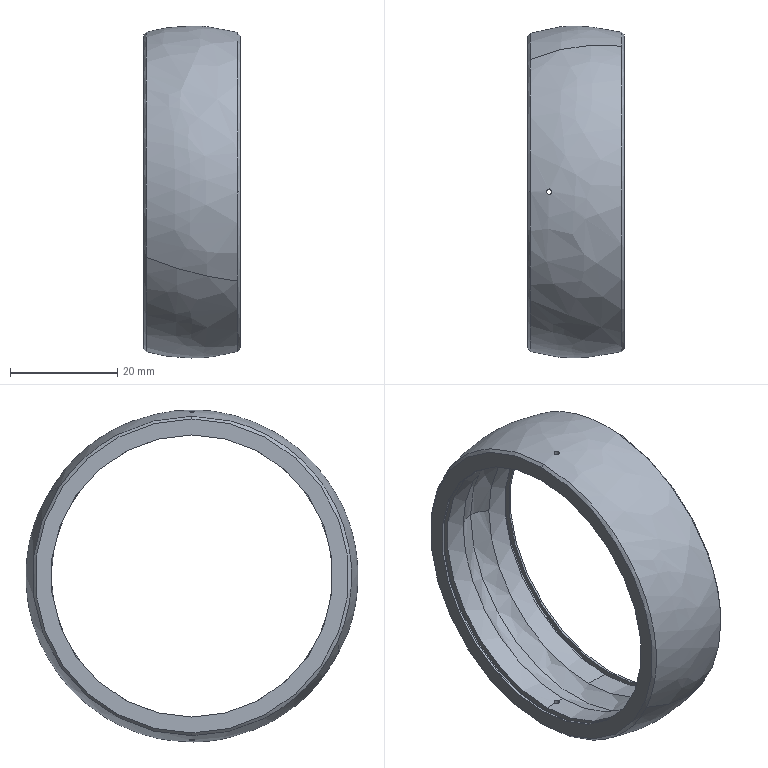Part | SolidWorks | features BaseBody 1 | 1 solid | 32 faces | box 18 x 62 x 62 mm | volume 12092 mm3 | cylinder 16 | spline 6 | plane 6 | cone 4 | commonest cylinder face diameters 52.667 x8 1 x4 54.667 x4
STEP:
#1=CARTESIAN_POINT('',(-5.,62.5,12.31));
#2=VERTEX_POINT('',#1);
#3=CARTESIAN_POINT('',(-5.,63.5,12.31));
#4=VERTEX_POINT('',#3);
#5=CARTESIAN_POINT('',(-5.,62.5,12.31));
#6=CARTESIAN_POINT('',(-4.87,62.5,12.289));
#7=CARTESIAN_POINT('',(-4.741,62.552,12.268));
#8=CARTESIAN_POINT('',(-4.554,62.738,12.237));
#9=CARTESIAN_POINT('',(-4.5,62.867,12.228));
#10=CARTESIAN_POINT('',(-4.5,63.133,12.228));
#11=CARTESIAN_POINT('',(-4.555,63.263,12.237));
#12=CARTESIAN_POINT('',(-4.74,63.447,12.268));
#13=CARTESIAN_POINT('',(-4.87,63.5,12.289));
#14=CARTESIAN_POINT('',(-5.,63.5,12.31));
#15=B_SPLINE_CURVE_WITH_KNOTS('',3,(#5,#6,#7,#8,#9,#10,#11,#12,#13,#14),.UNSPECIFIED.,.F.,.F.,(4,2,2,2,4),(0.000787,0.00118,0.001574,0.001967,0.00236),.UNSPECIFIED.);
#16=EDGE_CURVE('',#2,#4,#15,.T.);
#17=ORIENTED_EDGE('',*,*,#16,.T.);
#18=CARTESIAN_POINT('',(-5.,63.5,12.31));
#19=CARTESIAN_POINT('',(-5.13,63.5,12.331));
#20=CARTESIAN_POINT('',(-5.259,63.448,12.352));
#21=CARTESIAN_POINT('',(-5.446,63.262,12.383));
#22=CARTESIAN_POINT('',(-5.5,63.133,12.392));
#23=CARTESIAN_POINT('',(-5.5,62.867,12.392));
#24=CARTESIAN_POINT('',(-5.445,62.737,12.383));
#25=CARTESIAN_POINT('',(-5.26,62.553,12.352));
#26=CARTESIAN_POINT('',(-5.13,62.5,12.331));
#27=CARTESIAN_POINT('',(-5.,62.5,12.31));
#28=B_SPLINE_CURVE_WITH_KNOTS('',3,(#18,#19,#20,#21,#22,#23,#24,#25,#26,#27),.UNSPECIFIED.,.F.,.F.,(4,2,2,2,4),(0.00236,0.002754,0.003147,0.003541,0.003934),.UNSPECIFIED.);
#29=EDGE_CURVE('',#4,#2,#28,.T.);
#30=ORIENTED_EDGE('',*,*,#29,.T.);
#31=EDGE_LOOP('',(#17,#30));
#32=FACE_BOUND('',#31,.T.);
#33=CARTESIAN_POINT('',(8.5,92.812,42.9));
#34=VERTEX_POINT('',#33);
#35=CARTESIAN_POINT('',(8.5,38.269,26.252));
#36=VERTEX_POINT('',#35);
#37=CARTESIAN_POINT('',(8.5,63.,42.9));
#38=DIRECTION('',(-1.,0.,0.));
#39=DIRECTION('',(0.,0.,1.));
#40=AXIS2_PLACEMENT_3D('',#37,#38,#39);
#41=CIRCLE('',#40,29.812);
#42=EDGE_CURVE('',#34,#36,#41,.T.);
#43=ORIENTED_EDGE('',*,*,#42,.T.);
#44=CARTESIAN_POINT('',(-8.5,35.801,30.694));
#45=VERTEX_POINT('',#44);
#46=CARTESIAN_POINT('',(0.,63.,42.9));
#47=DIRECTION('',(-0.2864,0.4654,-0.8375));
#48=DIRECTION('',(0.7936,0.605,0.06481));
#49=AXIS2_PLACEMENT_3D('',#46,#47,#48);
#50=CIRCLE('',#49,31.);
#51=EDGE_CURVE('',#36,#45,#50,.T.);
#52=ORIENTED_EDGE('',*,*,#51,.T.);
#53=CARTESIAN_POINT('',(-8.5,63.,13.088));
#54=VERTEX_POINT('',#53);
#55=CARTESIAN_POINT('',(-8.5,63.,42.9));
#56=DIRECTION('',(1.,0.,0.));
#57=DIRECTION('',(0.,1.,0.));
#58=AXIS2_PLACEMENT_3D('',#55,#56,#57);
#59=CIRCLE('',#58,29.812);
#60=EDGE_CURVE('',#45,#54,#59,.T.);
#61=ORIENTED_EDGE('',*,*,#60,.T.);
#62=CARTESIAN_POINT('',(-8.5,87.731,59.548));
#63=VERTEX_POINT('',#62);
#64=CARTESIAN_POINT('',(-8.5,63.,42.9));
#65=DIRECTION('',(1.,0.,0.));
#66=DIRECTION('',(0.,1.,0.));
#67=AXIS2_PLACEMENT_3D('',#64,#65,#66);
#68=CIRCLE('',#67,29.812);
#69=EDGE_CURVE('',#54,#63,#68,.T.);
#70=ORIENTED_EDGE('',*,*,#69,.T.);
#71=CARTESIAN_POINT('',(8.5,90.199,55.106));
#72=VERTEX_POINT('',#71);
#73=CARTESIAN_POINT('',(0.,63.,42.9));
#74=DIRECTION('',(0.2864,-0.4654,0.8375));
#75=DIRECTION('',(0.7936,0.605,0.06481));
#76=AXIS2_PLACEMENT_3D('',#73,#74,#75);
#77=CIRCLE('',#76,31.);
#78=EDGE_CURVE('',#72,#63,#77,.T.);
#79=ORIENTED_EDGE('',*,*,#78,.F.);
#80=CARTESIAN_POINT('',(8.5,63.,42.9));
#81=DIRECTION('',(-1.,0.,0.));
#82=DIRECTION('',(0.,0.,1.));
#83=AXIS2_PLACEMENT_3D('',#80,#81,#82);
#84=CIRCLE('',#83,29.812);
#85=EDGE_CURVE('',#72,#34,#84,.T.);
#86=ORIENTED_EDGE('',*,*,#85,.T.);
#87=EDGE_LOOP('',(#43,#52,#61,#70,#79,#86));
#88=FACE_OUTER_BOUND('',#87,.T.);
#89=CARTESIAN_POINT('',(29.685,66.413,34.646));
#90=CARTESIAN_POINT('',(19.256,83.361,4.143));
#91=CARTESIAN_POINT('',(-0.2971,106.892,23.903));
#92=CARTESIAN_POINT('',(10.133,89.943,54.406));
#93=CARTESIAN_POINT('',(28.979,46.842,24.013));
#94=CARTESIAN_POINT('',(8.22,80.575,-36.698));
#95=CARTESIAN_POINT('',(-30.696,127.408,2.631));
#96=CARTESIAN_POINT('',(-9.938,93.675,63.342));
#97=CARTESIAN_POINT('',(11.581,33.025,22.285));
#98=CARTESIAN_POINT('',(-9.478,67.245,-39.303));
#99=CARTESIAN_POINT('',(-48.957,114.755,0.5944));
#100=CARTESIAN_POINT('',(-27.898,80.535,62.182));
#101=CARTESIAN_POINT('',(-8.81,35.843,30.823));
#102=CARTESIAN_POINT('',(-19.903,53.869,-1.621));
#103=CARTESIAN_POINT('',(-40.7,78.897,19.396));
#104=CARTESIAN_POINT('',(-29.606,60.87,51.84));
#105=(BOUNDED_SURFACE()B_SPLINE_SURFACE(3,3,((#89,#90,#91,#92),(#93,#94,#95,#96),(#97,#98,#99,#100),(#101,#102,#103,#104)),.UNSPECIFIED.,.F.,.F.,.T.)B_SPLINE_SURFACE_WITH_KNOTS((4,4),(4,4),(0.,1.),(0.,1.),.UNSPECIFIED.)GEOMETRIC_REPRESENTATION_ITEM()RATIONAL_B_SPLINE_SURFACE(((1.,0.3333,0.3333,1.),(0.7375,0.2458,0.2458,0.7375),(0.7375,0.2458,0.2458,0.7375),(1.,0.3333,0.3333,1.)))REPRESENTATION_ITEM('')SURFACE());
#106=ADVANCED_FACE('',(#32,#88),#105,.T.);
#107=CARTESIAN_POINT('',(0.,90.763,42.9));
#108=VERTEX_POINT('',#107);
#109=CARTESIAN_POINT('',(0.,35.238,42.9));
#110=VERTEX_POINT('',#109);
#111=CARTESIAN_POINT('',(0.,63.,42.9));
#112=DIRECTION('',(-1.,0.,0.));
#113=DIRECTION('',(0.,-1.,0.));
#114=AXIS2_PLACEMENT_3D('',#111,#112,#113);
#115=CIRCLE('',#114,27.762);
#116=EDGE_CURVE('',#108,#110,#115,.T.);
#117=ORIENTED_EDGE('',*,*,#116,.F.);
#118=CARTESIAN_POINT('',(-3.401,89.334,42.9));
#119=VERTEX_POINT('',#118);
#120=CARTESIAN_POINT('',(0.,86.,42.9));
#121=DIRECTION('',(0.,0.,1.));
#122=DIRECTION('',(0.,1.,0.));
#123=AXIS2_PLACEMENT_3D('',#120,#121,#122);
#124=CIRCLE('',#123,4.762);
#125=EDGE_CURVE('',#108,#119,#124,.T.);
#126=ORIENTED_EDGE('',*,*,#125,.T.);
#127=CARTESIAN_POINT('',(-3.401,63.,16.566));
#128=VERTEX_POINT('',#127);
#129=CARTESIAN_POINT('',(-3.401,63.,42.9));
#130=DIRECTION('',(1.,0.,0.));
#131=DIRECTION('',(0.,0.,1.));
#132=AXIS2_PLACEMENT_3D('',#129,#130,#131);
#133=CIRCLE('',#132,26.334);
#134=EDGE_CURVE('',#128,#119,#133,.T.);
#135=ORIENTED_EDGE('',*,*,#134,.F.);
#136=CARTESIAN_POINT('',(-3.401,36.666,42.9));
#137=VERTEX_POINT('',#136);
#138=CARTESIAN_POINT('',(-3.401,63.,42.9));
#139=DIRECTION('',(1.,0.,0.));
#140=DIRECTION('',(0.,0.,1.));
#141=AXIS2_PLACEMENT_3D('',#138,#139,#140);
#142=CIRCLE('',#141,26.334);
#143=EDGE_CURVE('',#137,#128,#142,.T.);
#144=ORIENTED_EDGE('',*,*,#143,.F.);
#145=CARTESIAN_POINT('',(0.,40.,42.9));
#146=DIRECTION('',(0.,0.,-1.));
#147=DIRECTION('',(0.,-1.,0.));
#148=AXIS2_PLACEMENT_3D('',#145,#146,#147);
#149=CIRCLE('',#148,4.762);
#150=EDGE_CURVE('',#110,#137,#149,.T.);
#151=ORIENTED_EDGE('',*,*,#150,.F.);
#152=EDGE_LOOP('',(#117,#126,#135,#144,#151));
#153=FACE_OUTER_BOUND('',#152,.T.);
#154=CARTESIAN_POINT('',(0.,90.763,42.9));
#155=CARTESIAN_POINT('',(0.,90.763,-12.625));
#156=CARTESIAN_POINT('',(0.,35.238,-12.625));
#157=CARTESIAN_POINT('',(0.,35.237,42.9));
#158=CARTESIAN_POINT('',(-1.297,90.763,42.9));
#159=CARTESIAN_POINT('',(-1.297,90.763,-12.625));
#160=CARTESIAN_POINT('',(-1.297,35.238,-12.625));
#161=CARTESIAN_POINT('',(-1.297,35.237,42.9));
#162=CARTESIAN_POINT('',(-2.493,90.26,42.9));
#163=CARTESIAN_POINT('',(-2.493,90.26,-11.62));
#164=CARTESIAN_POINT('',(-2.493,35.74,-11.62));
#165=CARTESIAN_POINT('',(-2.493,35.74,42.9));
#166=CARTESIAN_POINT('',(-3.401,89.334,42.9));
#167=CARTESIAN_POINT('',(-3.401,89.334,-9.767));
#168=CARTESIAN_POINT('',(-3.401,36.666,-9.767));
#169=CARTESIAN_POINT('',(-3.401,36.666,42.9));
#170=(BOUNDED_SURFACE()B_SPLINE_SURFACE(3,3,((#154,#155,#156,#157),(#158,#159,#160,#161),(#162,#163,#164,#165),(#166,#167,#168,#169)),.UNSPECIFIED.,.F.,.F.,.F.)B_SPLINE_SURFACE_WITH_KNOTS((4,4),(4,4),(0.,1.),(0.,1.),.UNSPECIFIED.)GEOMETRIC_REPRESENTATION_ITEM()RATIONAL_B_SPLINE_SURFACE(((1.,0.3333,0.3333,1.),(0.948,0.316,0.316,0.948),(0.948,0.316,0.316,0.948),(1.,0.3333,0.3333,1.)))REPRESENTATION_ITEM('')SURFACE());
#171=ADVANCED_FACE('',(#153),#170,.T.);
#172=CARTESIAN_POINT('',(3.401,63.,16.566));
#173=VERTEX_POINT('',#172);
#174=CARTESIAN_POINT('',(3.401,89.334,42.9));
#175=VERTEX_POINT('',#174);
#176=CARTESIAN_POINT('',(3.401,63.,42.9));
#177=DIRECTION('',(1.,0.,0.));
#178=DIRECTION('',(0.,-1.,0.));
#179=AXIS2_PLACEMENT_3D('',#176,#177,#178);
#180=CIRCLE('',#179,26.334);
#181=EDGE_CURVE('',#173,#175,#180,.T.);
#182=ORIENTED_EDGE('',*,*,#181,.T.);
#183=CARTESIAN_POINT('',(0.,86.,42.9));
#184=DIRECTION('',(0.,0.,1.));
#185=DIRECTION('',(0.,1.,0.));
#186=AXIS2_PLACEMENT_3D('',#183,#184,#185);
#187=CIRCLE('',#186,4.762);
#188=EDGE_CURVE('',#175,#108,#187,.T.);
#189=ORIENTED_EDGE('',*,*,#188,.T.);
#190=ORIENTED_EDGE('',*,*,#116,.T.);
#191=CARTESIAN_POINT('',(3.401,36.666,42.9));
#192=VERTEX_POINT('',#191);
#193=CARTESIAN_POINT('',(0.,40.,42.9));
#194=DIRECTION('',(0.,0.,-1.));
#195=DIRECTION('',(0.,-1.,0.));
#196=AXIS2_PLACEMENT_3D('',#193,#194,#195);
#197=CIRCLE('',#196,4.762);
#198=EDGE_CURVE('',#192,#110,#197,.T.);
#199=ORIENTED_EDGE('',*,*,#198,.F.);
#200=CARTESIAN_POINT('',(3.401,63.,42.9));
#201=DIRECTION('',(1.,0.,0.));
#202=DIRECTION('',(0.,-1.,0.));
#203=AXIS2_PLACEMENT_3D('',#200,#201,#202);
#204=CIRCLE('',#203,26.334);
#205=EDGE_CURVE('',#192,#173,#204,.T.);
#206=ORIENTED_EDGE('',*,*,#205,.T.);
#207=EDGE_LOOP('',(#182,#189,#190,#199,#206));
#208=FACE_OUTER_BOUND('',#207,.T.);
#209=CARTESIAN_POINT('',(3.401,89.334,42.9));
#210=CARTESIAN_POINT('',(3.401,89.334,-9.767));
#211=CARTESIAN_POINT('',(3.401,36.666,-9.767));
#212=CARTESIAN_POINT('',(3.401,36.666,42.9));
#213=CARTESIAN_POINT('',(2.493,90.26,42.9));
#214=CARTESIAN_POINT('',(2.493,90.26,-11.62));
#215=CARTESIAN_POINT('',(2.493,35.74,-11.62));
#216=CARTESIAN_POINT('',(2.493,35.74,42.9));
#217=CARTESIAN_POINT('',(1.297,90.763,42.9));
#218=CARTESIAN_POINT('',(1.297,90.763,-12.625));
#219=CARTESIAN_POINT('',(1.297,35.237,-12.625));
#220=CARTESIAN_POINT('',(1.297,35.237,42.9));
#221=CARTESIAN_POINT('',(0.,90.763,42.9));
#222=CARTESIAN_POINT('',(0.,90.763,-12.625));
#223=CARTESIAN_POINT('',(0.,35.238,-12.625));
#224=CARTESIAN_POINT('',(0.,35.237,42.9));
#225=(BOUNDED_SURFACE()B_SPLINE_SURFACE(3,3,((#209,#210,#211,#212),(#213,#214,#215,#216),(#217,#218,#219,#220),(#221,#222,#223,#224)),.UNSPECIFIED.,.F.,.F.,.F.)B_SPLINE_SURFACE_WITH_KNOTS((4,4),(4,4),(0.,1.),(0.,1.),.UNSPECIFIED.)GEOMETRIC_REPRESENTATION_ITEM()RATIONAL_B_SPLINE_SURFACE(((1.,0.3333,0.3333,1.),(0.948,0.316,0.316,0.948),(0.948,0.316,0.316,0.948),(1.,0.3333,0.3333,1.)))REPRESENTATION_ITEM('')SURFACE());
#226=ADVANCED_FACE('',(#208),#225,.T.);
#227=CARTESIAN_POINT('',(-5.,63.5,69.229));
#228=VERTEX_POINT('',#227);
#229=CARTESIAN_POINT('',(-5.5,63.,69.234));
#230=VERTEX_POINT('',#229);
#231=CARTESIAN_POINT('',(-5.,63.5,69.229));
#232=CARTESIAN_POINT('',(-5.132,63.5,69.229));
#233=CARTESIAN_POINT('',(-5.261,63.446,69.23));
#234=CARTESIAN_POINT('',(-5.446,63.262,69.233));
#235=CARTESIAN_POINT('',(-5.5,63.132,69.234));
#236=CARTESIAN_POINT('',(-5.5,63.,69.234));
#237=B_SPLINE_CURVE_WITH_KNOTS('',3,(#231,#232,#233,#234,#235,#236),.UNSPECIFIED.,.F.,.F.,(4,2,4),(0.,0.0003905,0.0007811),.UNSPECIFIED.);
#238=EDGE_CURVE('',#228,#230,#237,.T.);
#239=ORIENTED_EDGE('',*,*,#238,.F.);
#240=CARTESIAN_POINT('',(-5.,63.5,73.49));
#241=VERTEX_POINT('',#240);
#242=CARTESIAN_POINT('',(-5.,63.5,71.565));
#243=DIRECTION('',(0.,0.,1.));
#244=VECTOR('',#243,1000.);
#245=LINE('',#242,#244);
#246=EDGE_CURVE('',#228,#241,#245,.T.);
#247=ORIENTED_EDGE('',*,*,#246,.T.);
#248=CARTESIAN_POINT('',(-5.,62.5,73.49));
#249=VERTEX_POINT('',#248);
#250=CARTESIAN_POINT('',(-5.,62.5,73.49));
#251=CARTESIAN_POINT('',(-5.13,62.5,73.469));
#252=CARTESIAN_POINT('',(-5.259,62.552,73.448));
#253=CARTESIAN_POINT('',(-5.446,62.738,73.417));
#254=CARTESIAN_POINT('',(-5.5,62.867,73.408));
#255=CARTESIAN_POINT('',(-5.5,63.133,73.408));
#256=CARTESIAN_POINT('',(-5.445,63.263,73.417));
#257=CARTESIAN_POINT('',(-5.26,63.447,73.448));
#258=CARTESIAN_POINT('',(-5.13,63.5,73.469));
#259=CARTESIAN_POINT('',(-5.,63.5,73.49));
#260=B_SPLINE_CURVE_WITH_KNOTS('',3,(#250,#251,#252,#253,#254,#255,#256,#257,#258,#259),.UNSPECIFIED.,.F.,.F.,(4,2,2,2,4),(0.000787,0.00118,0.001574,0.001967,0.00236),.UNSPECIFIED.);
#261=EDGE_CURVE('',#249,#241,#260,.T.);
#262=ORIENTED_EDGE('',*,*,#261,.F.);
#263=CARTESIAN_POINT('',(-5.,62.5,69.229));
#264=VERTEX_POINT('',#263);
#265=CARTESIAN_POINT('',(-5.,62.5,71.565));
#266=DIRECTION('',(0.,0.,1.));
#267=VECTOR('',#266,1000.);
#268=LINE('',#265,#267);
#269=EDGE_CURVE('',#264,#249,#268,.T.);
#270=ORIENTED_EDGE('',*,*,#269,.F.);
#271=CARTESIAN_POINT('',(-5.5,63.,69.234));
#272=CARTESIAN_POINT('',(-5.5,62.868,69.234));
#273=CARTESIAN_POINT('',(-5.446,62.739,69.233));
#274=CARTESIAN_POINT('',(-5.262,62.554,69.23));
#275=CARTESIAN_POINT('',(-5.132,62.5,69.229));
#276=CARTESIAN_POINT('',(-5.,62.5,69.229));
#277=B_SPLINE_CURVE_WITH_KNOTS('',3,(#271,#272,#273,#274,#275,#276),.UNSPECIFIED.,.F.,.F.,(4,2,4),(0.0007811,0.001172,0.001562),.UNSPECIFIED.);
#278=EDGE_CURVE('',#230,#264,#277,.T.);
#279=ORIENTED_EDGE('',*,*,#278,.F.);
#280=EDGE_LOOP('',(#239,#247,#262,#270,#279));
#281=FACE_OUTER_BOUND('',#280,.T.);
#282=CARTESIAN_POINT('',(-5.,63.,71.565));
#283=DIRECTION('',(0.,0.,1.));
#284=DIRECTION('',(0.,-1.,0.));
#285=AXIS2_PLACEMENT_3D('',#282,#283,#284);
#286=CYLINDRICAL_SURFACE('',#285,0.5);
#287=ADVANCED_FACE('',(#281),#286,.F.);
#288=CARTESIAN_POINT('',(-9.,63.,13.588));
#289=VERTEX_POINT('',#288);
#290=CARTESIAN_POINT('',(-9.,63.,72.212));
#291=VERTEX_POINT('',#290);
#292=CARTESIAN_POINT('',(-9.,63.,42.9));
#293=DIRECTION('',(1.,0.,0.));
#294=DIRECTION('',(0.,0.,-1.));
#295=AXIS2_PLACEMENT_3D('',#292,#293,#294);
#296=CIRCLE('',#295,29.312);
#297=EDGE_CURVE('',#289,#291,#296,.T.);
#298=ORIENTED_EDGE('',*,*,#297,.T.);
#299=CARTESIAN_POINT('',(-8.5,63.,72.712));
#300=VERTEX_POINT('',#299);
#301=CARTESIAN_POINT('',(-8.5,63.,72.712));
#302=DIRECTION('',(0.7071,0.,0.7071));
#303=VECTOR('',#302,1000.);
#304=LINE('',#301,#303);
#305=EDGE_CURVE('',#291,#300,#304,.T.);
#306=ORIENTED_EDGE('',*,*,#305,.T.);
#307=CARTESIAN_POINT('',(-8.5,63.,42.9));
#308=DIRECTION('',(1.,0.,0.));
#309=DIRECTION('',(0.,1.,0.));
#310=AXIS2_PLACEMENT_3D('',#307,#308,#309);
#311=CIRCLE('',#310,29.812);
#312=EDGE_CURVE('',#63,#300,#311,.T.);
#313=ORIENTED_EDGE('',*,*,#312,.F.);
#314=ORIENTED_EDGE('',*,*,#69,.F.);
#315=CARTESIAN_POINT('',(-8.5,63.,13.088));
#316=DIRECTION('',(0.7071,0.,-0.7071));
#317=VECTOR('',#316,1000.);
#318=LINE('',#315,#317);
#319=EDGE_CURVE('',#289,#54,#318,.T.);
#320=ORIENTED_EDGE('',*,*,#319,.F.);
#321=EDGE_LOOP('',(#298,#306,#313,#314,#320));
#322=FACE_OUTER_BOUND('',#321,.T.);
#323=CARTESIAN_POINT('',(-8.5,63.,42.9));
#324=DIRECTION('',(1.,0.,0.));
#325=DIRECTION('',(0.,0.,-1.));
#326=AXIS2_PLACEMENT_3D('',#323,#324,#325);
#327=CONICAL_SURFACE('',#326,29.812,0.7854);
#328=ADVANCED_FACE('',(#322),#327,.T.);
#329=CARTESIAN_POINT('',(9.,33.688,42.9));
#330=VERTEX_POINT('',#329);
#331=CARTESIAN_POINT('',(9.,92.312,42.9));
#332=VERTEX_POINT('',#331);
#333=CARTESIAN_POINT('',(9.,63.,42.9));
#334=DIRECTION('',(-1.,0.,0.));
#335=DIRECTION('',(0.,-1.,0.));
#336=AXIS2_PLACEMENT_3D('',#333,#334,#335);
#337=CIRCLE('',#336,29.312);
#338=EDGE_CURVE('',#330,#332,#337,.T.);
#339=ORIENTED_EDGE('',*,*,#338,.T.);
#340=CARTESIAN_POINT('',(8.5,92.812,42.9));
#341=DIRECTION('',(-0.7071,0.7071,0.));
#342=VECTOR('',#341,1000.);
#343=LINE('',#340,#342);
#344=EDGE_CURVE('',#332,#34,#343,.T.);
#345=ORIENTED_EDGE('',*,*,#344,.T.);
#346=ORIENTED_EDGE('',*,*,#85,.F.);
#347=CARTESIAN_POINT('',(8.5,33.188,42.9));
#348=VERTEX_POINT('',#347);
#349=CARTESIAN_POINT('',(8.5,63.,42.9));
#350=DIRECTION('',(-1.,0.,0.));
#351=DIRECTION('',(0.,0.,1.));
#352=AXIS2_PLACEMENT_3D('',#349,#350,#351);
#353=CIRCLE('',#352,29.812);
#354=EDGE_CURVE('',#348,#72,#353,.T.);
#355=ORIENTED_EDGE('',*,*,#354,.F.);
#356=CARTESIAN_POINT('',(8.5,33.188,42.9));
#357=DIRECTION('',(-0.7071,-0.7071,0.));
#358=VECTOR('',#357,1000.);
#359=LINE('',#356,#358);
#360=EDGE_CURVE('',#330,#348,#359,.T.);
#361=ORIENTED_EDGE('',*,*,#360,.F.);
#362=EDGE_LOOP('',(#339,#345,#346,#355,#361));
#363=FACE_OUTER_BOUND('',#362,.T.);
#364=CARTESIAN_POINT('',(8.5,63.,42.9));
#365=DIRECTION('',(-1.,0.,0.));
#366=DIRECTION('',(0.,-1.,0.));
#367=AXIS2_PLACEMENT_3D('',#364,#365,#366);
#368=CONICAL_SURFACE('',#367,29.812,0.7854);
#369=ADVANCED_FACE('',(#363),#368,.T.);
#370=CARTESIAN_POINT('',(-3.401,63.,69.234));
#371=VERTEX_POINT('',#370);
#372=CARTESIAN_POINT('',(-3.401,63.,42.9));
#373=DIRECTION('',(1.,0.,0.));
#374=DIRECTION('',(0.,0.,1.));
#375=AXIS2_PLACEMENT_3D('',#372,#373,#374);
#376=CIRCLE('',#375,26.334);
#377=EDGE_CURVE('',#371,#137,#376,.T.);
#378=ORIENTED_EDGE('',*,*,#377,.T.);
#379=ORIENTED_EDGE('',*,*,#143,.T.);
#380=CARTESIAN_POINT('',(-4.5,63.,16.566));
#381=VERTEX_POINT('',#380);
#382=CARTESIAN_POINT('',(-3.401,63.,16.566));
#383=DIRECTION('',(-1.,0.,0.));
#384=VECTOR('',#383,1000.);
#385=LINE('',#382,#384);
#386=EDGE_CURVE('',#128,#381,#385,.T.);
#387=ORIENTED_EDGE('',*,*,#386,.T.);
#388=CARTESIAN_POINT('',(-5.,62.5,16.571));
#389=VERTEX_POINT('',#388);
#390=CARTESIAN_POINT('',(-4.5,63.,16.566));
#391=CARTESIAN_POINT('',(-4.5,62.868,16.566));
#392=CARTESIAN_POINT('',(-4.554,62.739,16.567));
#393=CARTESIAN_POINT('',(-4.738,62.554,16.57));
#394=CARTESIAN_POINT('',(-4.868,62.5,16.571));
#395=CARTESIAN_POINT('',(-5.,62.5,16.571));
#396=B_SPLINE_CURVE_WITH_KNOTS('',3,(#390,#391,#392,#393,#394,#395),.UNSPECIFIED.,.F.,.F.,(4,2,4),(0.0007811,0.001172,0.001562),.UNSPECIFIED.);
#397=EDGE_CURVE('',#381,#389,#396,.T.);
#398=ORIENTED_EDGE('',*,*,#397,.T.);
#399=CARTESIAN_POINT('',(-5.5,63.,16.566));
#400=VERTEX_POINT('',#399);
#401=CARTESIAN_POINT('',(-5.,62.5,16.571));
#402=CARTESIAN_POINT('',(-5.132,62.5,16.571));
#403=CARTESIAN_POINT('',(-5.261,62.554,16.57));
#404=CARTESIAN_POINT('',(-5.446,62.738,16.567));
#405=CARTESIAN_POINT('',(-5.5,62.868,16.566));
#406=CARTESIAN_POINT('',(-5.5,63.,16.566));
#407=B_SPLINE_CURVE_WITH_KNOTS('',3,(#401,#402,#403,#404,#405,#406),.UNSPECIFIED.,.F.,.F.,(4,2,4),(-0.001562,-0.001172,-0.0007811),.UNSPECIFIED.);
#408=EDGE_CURVE('',#389,#400,#407,.T.);
#409=ORIENTED_EDGE('',*,*,#408,.T.);
#410=CARTESIAN_POINT('',(-7.6,63.,16.566));
#411=VERTEX_POINT('',#410);
#412=CARTESIAN_POINT('',(-3.401,63.,16.566));
#413=DIRECTION('',(-1.,0.,0.));
#414=VECTOR('',#413,1000.);
#415=LINE('',#412,#414);
#416=EDGE_CURVE('',#400,#411,#415,.T.);
#417=ORIENTED_EDGE('',*,*,#416,.T.);
#418=CARTESIAN_POINT('',(-7.6,63.,69.234));
#419=VERTEX_POINT('',#418);
#420=CARTESIAN_POINT('',(-7.6,63.,42.9));
#421=DIRECTION('',(-1.,0.,0.));
#422=DIRECTION('',(0.,0.,1.));
#423=AXIS2_PLACEMENT_3D('',#420,#421,#422);
#424=CIRCLE('',#423,26.334);
#425=EDGE_CURVE('',#411,#419,#424,.T.);
#426=ORIENTED_EDGE('',*,*,#425,.T.);
#427=CARTESIAN_POINT('',(-3.401,63.,69.234));
#428=DIRECTION('',(-1.,0.,0.));
#429=VECTOR('',#428,1000.);
#430=LINE('',#427,#429);
#431=EDGE_CURVE('',#230,#419,#430,.T.);
#432=ORIENTED_EDGE('',*,*,#431,.F.);
#433=ORIENTED_EDGE('',*,*,#278,.T.);
#434=CARTESIAN_POINT('',(-4.5,63.,69.234));
#435=VERTEX_POINT('',#434);
#436=CARTESIAN_POINT('',(-5.,62.5,69.229));
#437=CARTESIAN_POINT('',(-4.868,62.5,69.229));
#438=CARTESIAN_POINT('',(-4.739,62.554,69.23));
#439=CARTESIAN_POINT('',(-4.554,62.738,69.233));
#440=CARTESIAN_POINT('',(-4.5,62.868,69.234));
#441=CARTESIAN_POINT('',(-4.5,63.,69.234));
#442=B_SPLINE_CURVE_WITH_KNOTS('',3,(#436,#437,#438,#439,#440,#441),.UNSPECIFIED.,.F.,.F.,(4,2,4),(0.001562,0.001953,0.002343),.UNSPECIFIED.);
#443=EDGE_CURVE('',#264,#435,#442,.T.);
#444=ORIENTED_EDGE('',*,*,#443,.T.);
#445=CARTESIAN_POINT('',(-3.401,63.,69.234));
#446=DIRECTION('',(-1.,0.,0.));
#447=VECTOR('',#446,1000.);
#448=LINE('',#445,#447);
#449=EDGE_CURVE('',#371,#435,#448,.T.);
#450=ORIENTED_EDGE('',*,*,#449,.F.);
#451=EDGE_LOOP('',(#378,#379,#387,#398,#409,#417,#426,#432,#433,#444,#450));
#452=FACE_OUTER_BOUND('',#451,.T.);
#453=CARTESIAN_POINT('',(-3.401,63.,42.9));
#454=DIRECTION('',(-1.,0.,0.));
#455=DIRECTION('',(0.,0.,1.));
#456=AXIS2_PLACEMENT_3D('',#453,#454,#455);
#457=CYLINDRICAL_SURFACE('',#456,26.334);
#458=ADVANCED_FACE('',(#452),#457,.F.);
#459=ORIENTED_EDGE('',*,*,#29,.F.);
#460=CARTESIAN_POINT('',(-5.,63.5,16.571));
#461=VERTEX_POINT('',#460);
#462=CARTESIAN_POINT('',(-5.,63.5,14.235));
#463=DIRECTION('',(0.,0.,1.));
#464=VECTOR('',#463,1000.);
#465=LINE('',#462,#464);
#466=EDGE_CURVE('',#4,#461,#465,.T.);
#467=ORIENTED_EDGE('',*,*,#466,.T.);
#468=CARTESIAN_POINT('',(-5.5,63.,16.566));
#469=CARTESIAN_POINT('',(-5.5,63.132,16.566));
#470=CARTESIAN_POINT('',(-5.446,63.261,16.567));
#471=CARTESIAN_POINT('',(-5.262,63.446,16.57));
#472=CARTESIAN_POINT('',(-5.132,63.5,16.571));
#473=CARTESIAN_POINT('',(-5.,63.5,16.571));
#474=B_SPLINE_CURVE_WITH_KNOTS('',3,(#468,#469,#470,#471,#472,#473),.UNSPECIFIED.,.F.,.F.,(4,2,4),(-0.0007811,-0.0003905,0.),.UNSPECIFIED.);
#475=EDGE_CURVE('',#400,#461,#474,.T.);
#476=ORIENTED_EDGE('',*,*,#475,.F.);
#477=ORIENTED_EDGE('',*,*,#408,.F.);
#478=CARTESIAN_POINT('',(-5.,62.5,14.235));
#479=DIRECTION('',(0.,0.,1.));
#480=VECTOR('',#479,1000.);
#481=LINE('',#478,#480);
#482=EDGE_CURVE('',#2,#389,#481,.T.);
#483=ORIENTED_EDGE('',*,*,#482,.F.);
#484=EDGE_LOOP('',(#459,#467,#476,#477,#483));
#485=FACE_OUTER_BOUND('',#484,.T.);
#486=CARTESIAN_POINT('',(-5.,63.,14.235));
#487=DIRECTION('',(0.,0.,1.));
#488=DIRECTION('',(0.,-1.,0.));
#489=AXIS2_PLACEMENT_3D('',#486,#487,#488);
#490=CYLINDRICAL_SURFACE('',#489,0.5);
#491=ADVANCED_FACE('',(#485),#490,.F.);
#492=ORIENTED_EDGE('',*,*,#188,.F.);
#493=CARTESIAN_POINT('',(3.401,63.,69.234));
#494=VERTEX_POINT('',#493);
#495=CARTESIAN_POINT('',(3.401,63.,42.9));
#496=DIRECTION('',(1.,0.,0.));
#497=DIRECTION('',(0.,-1.,0.));
#498=AXIS2_PLACEMENT_3D('',#495,#496,#497);
#499=CIRCLE('',#498,26.334);
#500=EDGE_CURVE('',#175,#494,#499,.T.);
#501=ORIENTED_EDGE('',*,*,#500,.T.);
#502=CARTESIAN_POINT('',(3.401,63.,42.9));
#503=DIRECTION('',(1.,0.,0.));
#504=DIRECTION('',(0.,-1.,0.));
#505=AXIS2_PLACEMENT_3D('',#502,#503,#504);
#506=CIRCLE('',#505,26.334);
#507=EDGE_CURVE('',#494,#192,#506,.T.);
#508=ORIENTED_EDGE('',*,*,#507,.T.);
#509=ORIENTED_EDGE('',*,*,#198,.T.);
#510=CARTESIAN_POINT('',(0.,63.,42.9));
#511=DIRECTION('',(-1.,0.,0.));
#512=DIRECTION('',(0.,-1.,0.));
#513=AXIS2_PLACEMENT_3D('',#510,#511,#512);
#514=CIRCLE('',#513,27.762);
#515=EDGE_CURVE('',#110,#108,#514,.T.);
#516=ORIENTED_EDGE('',*,*,#515,.T.);
#517=EDGE_LOOP('',(#492,#501,#508,#509,#516));
#518=FACE_OUTER_BOUND('',#517,.T.);
#519=CARTESIAN_POINT('',(3.401,36.666,42.9));
#520=CARTESIAN_POINT('',(3.401,36.666,95.567));
#521=CARTESIAN_POINT('',(3.401,89.334,95.567));
#522=CARTESIAN_POINT('',(3.401,89.334,42.9));
#523=CARTESIAN_POINT('',(2.493,35.74,42.9));
#524=CARTESIAN_POINT('',(2.493,35.74,97.42));
#525=CARTESIAN_POINT('',(2.493,90.26,97.42));
#526=CARTESIAN_POINT('',(2.493,90.26,42.9));
#527=CARTESIAN_POINT('',(1.297,35.237,42.9));
#528=CARTESIAN_POINT('',(1.297,35.237,98.425));
#529=CARTESIAN_POINT('',(1.297,90.762,98.425));
#530=CARTESIAN_POINT('',(1.297,90.762,42.9));
#531=CARTESIAN_POINT('',(0.,35.237,42.9));
#532=CARTESIAN_POINT('',(0.,35.237,98.425));
#533=CARTESIAN_POINT('',(0.,90.762,98.425));
#534=CARTESIAN_POINT('',(0.,90.763,42.9));
#535=(BOUNDED_SURFACE()B_SPLINE_SURFACE(3,3,((#519,#520,#521,#522),(#523,#524,#525,#526),(#527,#528,#529,#530),(#531,#532,#533,#534)),.UNSPECIFIED.,.F.,.F.,.F.)B_SPLINE_SURFACE_WITH_KNOTS((4,4),(4,4),(0.,1.),(0.,1.),.UNSPECIFIED.)GEOMETRIC_REPRESENTATION_ITEM()RATIONAL_B_SPLINE_SURFACE(((1.,0.3333,0.3333,1.),(0.948,0.316,0.316,0.948),(0.948,0.316,0.316,0.948),(1.,0.3333,0.3333,1.)))REPRESENTATION_ITEM('')SURFACE());
#536=ADVANCED_FACE('',(#518),#535,.T.);
#537=CARTESIAN_POINT('',(-8.6,63.,69.234));
#538=VERTEX_POINT('',#537);
#539=CARTESIAN_POINT('',(-8.6,63.,16.566));
#540=VERTEX_POINT('',#539);
#541=CARTESIAN_POINT('',(-8.6,63.,42.9));
#542=DIRECTION('',(1.,0.,0.));
#543=DIRECTION('',(0.,0.,1.));
#544=AXIS2_PLACEMENT_3D('',#541,#542,#543);
#545=CIRCLE('',#544,26.334);
#546=EDGE_CURVE('',#538,#540,#545,.T.);
#547=ORIENTED_EDGE('',*,*,#546,.T.);
#548=CARTESIAN_POINT('',(-9.,63.,16.566));
#549=VERTEX_POINT('',#548);
#550=CARTESIAN_POINT('',(-8.6,63.,16.566));
#551=DIRECTION('',(-1.,0.,0.));
#552=VECTOR('',#551,1000.);
#553=LINE('',#550,#552);
#554=EDGE_CURVE('',#540,#549,#553,.T.);
#555=ORIENTED_EDGE('',*,*,#554,.T.);
#556=CARTESIAN_POINT('',(-9.,63.,69.234));
#557=VERTEX_POINT('',#556);
#558=CARTESIAN_POINT('',(-9.,63.,42.9));
#559=DIRECTION('',(1.,0.,0.));
#560=DIRECTION('',(0.,0.,1.));
#561=AXIS2_PLACEMENT_3D('',#558,#559,#560);
#562=CIRCLE('',#561,26.334);
#563=EDGE_CURVE('',#557,#549,#562,.T.);
#564=ORIENTED_EDGE('',*,*,#563,.F.);
#565=CARTESIAN_POINT('',(-8.6,63.,69.234));
#566=DIRECTION('',(-1.,0.,0.));
#567=VECTOR('',#566,1000.);
#568=LINE('',#565,#567);
#569=EDGE_CURVE('',#538,#557,#568,.T.);
#570=ORIENTED_EDGE('',*,*,#569,.F.);
#571=EDGE_LOOP('',(#547,#555,#564,#570));
#572=FACE_OUTER_BOUND('',#571,.T.);
#573=CARTESIAN_POINT('',(-8.6,63.,42.9));
#574=DIRECTION('',(-1.,0.,0.));
#575=DIRECTION('',(0.,0.,1.));
#576=AXIS2_PLACEMENT_3D('',#573,#574,#575);
#577=CYLINDRICAL_SURFACE('',#576,26.334);
#578=ADVANCED_FACE('',(#572),#577,.F.);
#579=CARTESIAN_POINT('',(9.,63.,16.566));
#580=VERTEX_POINT('',#579);
#581=CARTESIAN_POINT('',(9.,63.,69.234));
#582=VERTEX_POINT('',#581);
#583=CARTESIAN_POINT('',(9.,63.,42.9));
#584=DIRECTION('',(-1.,0.,0.));
#585=DIRECTION('',(0.,0.,1.));
#586=AXIS2_PLACEMENT_3D('',#583,#584,#585);
#587=CIRCLE('',#586,26.334);
#588=EDGE_CURVE('',#580,#582,#587,.T.);
#589=ORIENTED_EDGE('',*,*,#588,.F.);
#590=CARTESIAN_POINT('',(8.6,63.,16.566));
#591=VERTEX_POINT('',#590);
#592=CARTESIAN_POINT('',(9.,63.,16.566));
#593=DIRECTION('',(-1.,0.,0.));
#594=VECTOR('',#593,1000.);
#595=LINE('',#592,#594);
#596=EDGE_CURVE('',#580,#591,#595,.T.);
#597=ORIENTED_EDGE('',*,*,#596,.T.);
#598=CARTESIAN_POINT('',(8.6,63.,69.234));
#599=VERTEX_POINT('',#598);
#600=CARTESIAN_POINT('',(8.6,63.,42.9));
#601=DIRECTION('',(-1.,0.,0.));
#602=DIRECTION('',(0.,0.,1.));
#603=AXIS2_PLACEMENT_3D('',#600,#601,#602);
#604=CIRCLE('',#603,26.334);
#605=EDGE_CURVE('',#591,#599,#604,.T.);
#606=ORIENTED_EDGE('',*,*,#605,.T.);
#607=CARTESIAN_POINT('',(9.,63.,69.234));
#608=DIRECTION('',(-1.,0.,0.));
#609=VECTOR('',#608,1000.);
#610=LINE('',#607,#609);
#611=EDGE_CURVE('',#582,#599,#610,.T.);
#612=ORIENTED_EDGE('',*,*,#611,.F.);
#613=EDGE_LOOP('',(#589,#597,#606,#612));
#614=FACE_OUTER_BOUND('',#613,.T.);
#615=CARTESIAN_POINT('',(9.,63.,42.9));
#616=DIRECTION('',(-1.,0.,0.));
#617=DIRECTION('',(0.,0.,1.));
#618=AXIS2_PLACEMENT_3D('',#615,#616,#617);
#619=CYLINDRICAL_SURFACE('',#618,26.334);
#620=ADVANCED_FACE('',(#614),#619,.F.);
#621=CARTESIAN_POINT('',(7.6,63.,69.234));
#622=VERTEX_POINT('',#621);
#623=CARTESIAN_POINT('',(7.6,63.,16.566));
#624=VERTEX_POINT('',#623);
#625=CARTESIAN_POINT('',(7.6,63.,42.9));
#626=DIRECTION('',(1.,0.,0.));
#627=DIRECTION('',(0.,0.,1.));
#628=AXIS2_PLACEMENT_3D('',#625,#626,#627);
#629=CIRCLE('',#628,26.334);
#630=EDGE_CURVE('',#622,#624,#629,.T.);
#631=ORIENTED_EDGE('',*,*,#630,.T.);
#632=CARTESIAN_POINT('',(7.6,63.,16.566));
#633=DIRECTION('',(-1.,0.,0.));
#634=VECTOR('',#633,1000.);
#635=LINE('',#632,#634);
#636=EDGE_CURVE('',#624,#173,#635,.T.);
#637=ORIENTED_EDGE('',*,*,#636,.T.);
#638=ORIENTED_EDGE('',*,*,#205,.F.);
#639=ORIENTED_EDGE('',*,*,#507,.F.);
#640=CARTESIAN_POINT('',(7.6,63.,69.234));
#641=DIRECTION('',(-1.,0.,0.));
#642=VECTOR('',#641,1000.);
#643=LINE('',#640,#642);
#644=EDGE_CURVE('',#622,#494,#643,.T.);
#645=ORIENTED_EDGE('',*,*,#644,.F.);
#646=EDGE_LOOP('',(#631,#637,#638,#639,#645));
#647=FACE_OUTER_BOUND('',#646,.T.);
#648=CARTESIAN_POINT('',(7.6,63.,42.9));
#649=DIRECTION('',(-1.,0.,0.));
#650=DIRECTION('',(0.,0.,1.));
#651=AXIS2_PLACEMENT_3D('',#648,#649,#650);
#652=CYLINDRICAL_SURFACE('',#651,26.334);
#653=ADVANCED_FACE('',(#647),#652,.F.);
#654=CARTESIAN_POINT('',(-7.6,63.,15.566));
#655=VERTEX_POINT('',#654);
#656=CARTESIAN_POINT('',(-7.6,63.,70.234));
#657=VERTEX_POINT('',#656);
#658=CARTESIAN_POINT('',(-7.6,63.,42.9));
#659=DIRECTION('',(-1.,0.,0.));
#660=DIRECTION('',(0.,0.,1.));
#661=AXIS2_PLACEMENT_3D('',#658,#659,#660);
#662=CIRCLE('',#661,27.334);
#663=EDGE_CURVE('',#655,#657,#662,.T.);
#664=ORIENTED_EDGE('',*,*,#663,.F.);
#665=CARTESIAN_POINT('',(-8.6,63.,15.566));
#666=VERTEX_POINT('',#665);
#667=CARTESIAN_POINT('',(-7.6,63.,15.566));
#668=DIRECTION('',(-1.,0.,0.));
#669=VECTOR('',#668,1000.);
#670=LINE('',#667,#669);
#671=EDGE_CURVE('',#655,#666,#670,.T.);
#672=ORIENTED_EDGE('',*,*,#671,.T.);
#673=CARTESIAN_POINT('',(-8.6,63.,70.234));
#674=VERTEX_POINT('',#673);
#675=CARTESIAN_POINT('',(-8.6,63.,42.9));
#676=DIRECTION('',(-1.,0.,0.));
#677=DIRECTION('',(0.,0.,1.));
#678=AXIS2_PLACEMENT_3D('',#675,#676,#677);
#679=CIRCLE('',#678,27.334);
#680=EDGE_CURVE('',#666,#674,#679,.T.);
#681=ORIENTED_EDGE('',*,*,#680,.T.);
#682=CARTESIAN_POINT('',(-7.6,63.,70.234));
#683=DIRECTION('',(-1.,0.,0.));
#684=VECTOR('',#683,1000.);
#685=LINE('',#682,#684);
#686=EDGE_CURVE('',#657,#674,#685,.T.);
#687=ORIENTED_EDGE('',*,*,#686,.F.);
#688=EDGE_LOOP('',(#664,#672,#681,#687));
#689=FACE_OUTER_BOUND('',#688,.T.);
#690=CARTESIAN_POINT('',(-7.6,63.,42.9));
#691=DIRECTION('',(-1.,0.,0.));
#692=DIRECTION('',(0.,0.,1.));
#693=AXIS2_PLACEMENT_3D('',#690,#691,#692);
#694=CYLINDRICAL_SURFACE('',#693,27.334);
#695=ADVANCED_FACE('',(#689),#694,.F.);
#696=CARTESIAN_POINT('',(8.6,63.,15.566));
#697=VERTEX_POINT('',#696);
#698=CARTESIAN_POINT('',(8.6,63.,70.234));
#699=VERTEX_POINT('',#698);
#700=CARTESIAN_POINT('',(8.6,63.,42.9));
#701=DIRECTION('',(-1.,0.,0.));
#702=DIRECTION('',(0.,0.,1.));
#703=AXIS2_PLACEMENT_3D('',#700,#701,#702);
#704=CIRCLE('',#703,27.334);
#705=EDGE_CURVE('',#697,#699,#704,.T.);
#706=ORIENTED_EDGE('',*,*,#705,.F.);
#707=CARTESIAN_POINT('',(7.6,63.,15.566));
#708=VERTEX_POINT('',#707);
#709=CARTESIAN_POINT('',(8.6,63.,15.566));
#710=DIRECTION('',(-1.,0.,0.));
#711=VECTOR('',#710,1000.);
#712=LINE('',#709,#711);
#713=EDGE_CURVE('',#697,#708,#712,.T.);
#714=ORIENTED_EDGE('',*,*,#713,.T.);
#715=CARTESIAN_POINT('',(7.6,63.,70.234));
#716=VERTEX_POINT('',#715);
#717=CARTESIAN_POINT('',(7.6,63.,42.9));
#718=DIRECTION('',(1.,0.,0.));
#719=DIRECTION('',(0.,0.,1.));
#720=AXIS2_PLACEMENT_3D('',#717,#718,#719);
#721=CIRCLE('',#720,27.334);
#722=EDGE_CURVE('',#716,#708,#721,.T.);
#723=ORIENTED_EDGE('',*,*,#722,.F.);
#724=CARTESIAN_POINT('',(8.6,63.,70.234));
#725=DIRECTION('',(-1.,0.,0.));
#726=VECTOR('',#725,1000.);
#727=LINE('',#724,#726);
#728=EDGE_CURVE('',#699,#716,#727,.T.);
#729=ORIENTED_EDGE('',*,*,#728,.F.);
#730=EDGE_LOOP('',(#706,#714,#723,#729));
#731=FACE_OUTER_BOUND('',#730,.T.);
#732=CARTESIAN_POINT('',(8.6,63.,42.9));
#733=DIRECTION('',(-1.,0.,0.));
#734=DIRECTION('',(0.,0.,1.));
#735=AXIS2_PLACEMENT_3D('',#732,#733,#734);
#736=CYLINDRICAL_SURFACE('',#735,27.334);
#737=ADVANCED_FACE('',(#731),#736,.F.);
#738=ORIENTED_EDGE('',*,*,#51,.F.);
#739=CARTESIAN_POINT('',(8.5,63.,42.9));
#740=DIRECTION('',(-1.,0.,0.));
#741=DIRECTION('',(0.,0.,1.));
#742=AXIS2_PLACEMENT_3D('',#739,#740,#741);
#743=CIRCLE('',#742,29.812);
#744=EDGE_CURVE('',#36,#348,#743,.T.);
#745=ORIENTED_EDGE('',*,*,#744,.T.);
#746=ORIENTED_EDGE('',*,*,#354,.T.);
#747=ORIENTED_EDGE('',*,*,#78,.T.);
#748=ORIENTED_EDGE('',*,*,#312,.T.);
#749=CARTESIAN_POINT('',(-8.5,63.,42.9));
#750=DIRECTION('',(1.,0.,0.));
#751=DIRECTION('',(0.,1.,0.));
#752=AXIS2_PLACEMENT_3D('',#749,#750,#751);
#753=CIRCLE('',#752,29.812);
#754=EDGE_CURVE('',#300,#45,#753,.T.);
#755=ORIENTED_EDGE('',*,*,#754,.T.);
#756=EDGE_LOOP('',(#738,#745,#746,#747,#748,#755));
#757=FACE_OUTER_BOUND('',#756,.T.);
#758=ORIENTED_EDGE('',*,*,#261,.T.);
#759=CARTESIAN_POINT('',(-5.,63.5,73.49));
#760=CARTESIAN_POINT('',(-4.87,63.5,73.511));
#761=CARTESIAN_POINT('',(-4.741,63.448,73.532));
#762=CARTESIAN_POINT('',(-4.554,63.262,73.563));
#763=CARTESIAN_POINT('',(-4.5,63.133,73.572));
#764=CARTESIAN_POINT('',(-4.5,62.867,73.572));
#765=CARTESIAN_POINT('',(-4.555,62.737,73.563));
#766=CARTESIAN_POINT('',(-4.74,62.553,73.532));
#767=CARTESIAN_POINT('',(-4.87,62.5,73.511));
#768=CARTESIAN_POINT('',(-5.,62.5,73.49));
#769=B_SPLINE_CURVE_WITH_KNOTS('',3,(#759,#760,#761,#762,#763,#764,#765,#766,#767,#768),.UNSPECIFIED.,.F.,.F.,(4,2,2,2,4),(0.00236,0.002754,0.003147,0.003541,0.003934),.UNSPECIFIED.);
#770=EDGE_CURVE('',#241,#249,#769,.T.);
#771=ORIENTED_EDGE('',*,*,#770,.T.);
#772=EDGE_LOOP('',(#758,#771));
#773=FACE_BOUND('',#772,.T.);
#774=CARTESIAN_POINT('',(8.811,90.157,54.977));
#775=CARTESIAN_POINT('',(19.904,72.131,87.419));
#776=CARTESIAN_POINT('',(40.699,47.105,66.402));
#777=CARTESIAN_POINT('',(29.607,65.131,33.961));
#778=CARTESIAN_POINT('',(-11.683,92.99,63.558));
#779=CARTESIAN_POINT('',(9.426,58.688,125.293));
#780=CARTESIAN_POINT('',(49.,11.064,85.301));
#781=CARTESIAN_POINT('',(27.891,45.366,23.566));
#782=CARTESIAN_POINT('',(-29.127,79.055,61.78));
#783=CARTESIAN_POINT('',(-8.363,45.313,122.507));
#784=CARTESIAN_POINT('',(30.564,-1.532,83.168));
#785=CARTESIAN_POINT('',(9.8,32.21,22.441));
#786=CARTESIAN_POINT('',(-29.691,59.402,51.053));
#787=CARTESIAN_POINT('',(-19.36,42.613,81.27));
#788=CARTESIAN_POINT('',(0.009585,19.303,61.695));
#789=CARTESIAN_POINT('',(-10.322,36.093,31.479));
#790=(BOUNDED_SURFACE()B_SPLINE_SURFACE(3,3,((#774,#775,#776,#777),(#778,#779,#780,#781),(#782,#783,#784,#785),(#786,#787,#788,#789)),.UNSPECIFIED.,.F.,.F.,.T.)B_SPLINE_SURFACE_WITH_KNOTS((4,4),(4,4),(0.,1.),(0.,1.),.UNSPECIFIED.)GEOMETRIC_REPRESENTATION_ITEM()RATIONAL_B_SPLINE_SURFACE(((1.,0.3333,0.3333,1.),(0.7357,0.2452,0.2452,0.7357),(0.7357,0.2452,0.2452,0.7357),(1.,0.3333,0.3333,1.)))REPRESENTATION_ITEM('')SURFACE());
#791=ADVANCED_FACE('',(#757,#773),#790,.T.);
#792=ORIENTED_EDGE('',*,*,#246,.F.);
#793=CARTESIAN_POINT('',(-4.5,63.,69.234));
#794=CARTESIAN_POINT('',(-4.5,63.132,69.234));
#795=CARTESIAN_POINT('',(-4.554,63.261,69.233));
#796=CARTESIAN_POINT('',(-4.738,63.446,69.23));
#797=CARTESIAN_POINT('',(-4.868,63.5,69.229));
#798=CARTESIAN_POINT('',(-5.,63.5,69.229));
#799=B_SPLINE_CURVE_WITH_KNOTS('',3,(#793,#794,#795,#796,#797,#798),.UNSPECIFIED.,.F.,.F.,(4,2,4),(-0.0007811,-0.0003905,0.),.UNSPECIFIED.);
#800=EDGE_CURVE('',#435,#228,#799,.T.);
#801=ORIENTED_EDGE('',*,*,#800,.F.);
#802=ORIENTED_EDGE('',*,*,#443,.F.);
#803=ORIENTED_EDGE('',*,*,#269,.T.);
#804=ORIENTED_EDGE('',*,*,#770,.F.);
#805=EDGE_LOOP('',(#792,#801,#802,#803,#804));
#806=FACE_OUTER_BOUND('',#805,.T.);
#807=CARTESIAN_POINT('',(-5.,63.,71.565));
#808=DIRECTION('',(0.,0.,1.));
#809=DIRECTION('',(0.,-1.,0.));
#810=AXIS2_PLACEMENT_3D('',#807,#808,#809);
#811=CYLINDRICAL_SURFACE('',#810,0.5);
#812=ADVANCED_FACE('',(#806),#811,.F.);
#813=ORIENTED_EDGE('',*,*,#305,.F.);
#814=CARTESIAN_POINT('',(-9.,63.,42.9));
#815=DIRECTION('',(1.,0.,0.));
#816=DIRECTION('',(0.,0.,-1.));
#817=AXIS2_PLACEMENT_3D('',#814,#815,#816);
#818=CIRCLE('',#817,29.312);
#819=EDGE_CURVE('',#291,#289,#818,.T.);
#820=ORIENTED_EDGE('',*,*,#819,.T.);
#821=ORIENTED_EDGE('',*,*,#319,.T.);
#822=ORIENTED_EDGE('',*,*,#60,.F.);
#823=ORIENTED_EDGE('',*,*,#754,.F.);
#824=EDGE_LOOP('',(#813,#820,#821,#822,#823));
#825=FACE_OUTER_BOUND('',#824,.T.);
#826=CARTESIAN_POINT('',(-8.5,63.,42.9));
#827=DIRECTION('',(1.,0.,0.));
#828=DIRECTION('',(0.,0.,-1.));
#829=AXIS2_PLACEMENT_3D('',#826,#827,#828);
#830=CONICAL_SURFACE('',#829,29.812,0.7854);
#831=ADVANCED_FACE('',(#825),#830,.T.);
#832=ORIENTED_EDGE('',*,*,#344,.F.);
#833=CARTESIAN_POINT('',(9.,63.,42.9));
#834=DIRECTION('',(-1.,0.,0.));
#835=DIRECTION('',(0.,-1.,0.));
#836=AXIS2_PLACEMENT_3D('',#833,#834,#835);
#837=CIRCLE('',#836,29.312);
#838=EDGE_CURVE('',#332,#330,#837,.T.);
#839=ORIENTED_EDGE('',*,*,#838,.T.);
#840=ORIENTED_EDGE('',*,*,#360,.T.);
#841=ORIENTED_EDGE('',*,*,#744,.F.);
#842=ORIENTED_EDGE('',*,*,#42,.F.);
#843=EDGE_LOOP('',(#832,#839,#840,#841,#842));
#844=FACE_OUTER_BOUND('',#843,.T.);
#845=CARTESIAN_POINT('',(8.5,63.,42.9));
#846=DIRECTION('',(-1.,0.,0.));
#847=DIRECTION('',(0.,-1.,0.));
#848=AXIS2_PLACEMENT_3D('',#845,#846,#847);
#849=CONICAL_SURFACE('',#848,29.812,0.7854);
#850=ADVANCED_FACE('',(#844),#849,.T.);
#851=ORIENTED_EDGE('',*,*,#386,.F.);
#852=ORIENTED_EDGE('',*,*,#134,.T.);
#853=CARTESIAN_POINT('',(-3.401,63.,42.9));
#854=DIRECTION('',(1.,0.,0.));
#855=DIRECTION('',(0.,0.,1.));
#856=AXIS2_PLACEMENT_3D('',#853,#854,#855);
#857=CIRCLE('',#856,26.334);
#858=EDGE_CURVE('',#119,#371,#857,.T.);
#859=ORIENTED_EDGE('',*,*,#858,.T.);
#860=ORIENTED_EDGE('',*,*,#449,.T.);
#861=ORIENTED_EDGE('',*,*,#800,.T.);
#862=ORIENTED_EDGE('',*,*,#238,.T.);
#863=ORIENTED_EDGE('',*,*,#431,.T.);
#864=CARTESIAN_POINT('',(-7.6,63.,42.9));
#865=DIRECTION('',(-1.,0.,0.));
#866=DIRECTION('',(0.,0.,1.));
#867=AXIS2_PLACEMENT_3D('',#864,#865,#866);
#868=CIRCLE('',#867,26.334);
#869=EDGE_CURVE('',#419,#411,#868,.T.);
#870=ORIENTED_EDGE('',*,*,#869,.T.);
#871=ORIENTED_EDGE('',*,*,#416,.F.);
#872=ORIENTED_EDGE('',*,*,#475,.T.);
#873=CARTESIAN_POINT('',(-5.,63.5,16.571));
#874=CARTESIAN_POINT('',(-4.868,63.5,16.571));
#875=CARTESIAN_POINT('',(-4.739,63.446,16.57));
#876=CARTESIAN_POINT('',(-4.554,63.262,16.567));
#877=CARTESIAN_POINT('',(-4.5,63.132,16.566));
#878=CARTESIAN_POINT('',(-4.5,63.,16.566));
#879=B_SPLINE_CURVE_WITH_KNOTS('',3,(#873,#874,#875,#876,#877,#878),.UNSPECIFIED.,.F.,.F.,(4,2,4),(0.,0.0003905,0.0007811),.UNSPECIFIED.);
#880=EDGE_CURVE('',#461,#381,#879,.T.);
#881=ORIENTED_EDGE('',*,*,#880,.T.);
#882=EDGE_LOOP('',(#851,#852,#859,#860,#861,#862,#863,#870,#871,#872,#881));
#883=FACE_OUTER_BOUND('',#882,.T.);
#884=CARTESIAN_POINT('',(-3.401,63.,42.9));
#885=DIRECTION('',(-1.,0.,0.));
#886=DIRECTION('',(0.,0.,1.));
#887=AXIS2_PLACEMENT_3D('',#884,#885,#886);
#888=CYLINDRICAL_SURFACE('',#887,26.334);
#889=ADVANCED_FACE('',(#883),#888,.F.);
#890=ORIENTED_EDGE('',*,*,#297,.F.);
#891=ORIENTED_EDGE('',*,*,#819,.F.);
#892=EDGE_LOOP('',(#890,#891));
#893=FACE_OUTER_BOUND('',#892,.T.);
#894=ORIENTED_EDGE('',*,*,#563,.T.);
#895=CARTESIAN_POINT('',(-9.,63.,42.9));
#896=DIRECTION('',(1.,0.,0.));
#897=DIRECTION('',(0.,0.,1.));
#898=AXIS2_PLACEMENT_3D('',#895,#896,#897);
#899=CIRCLE('',#898,26.334);
#900=EDGE_CURVE('',#549,#557,#899,.T.);
#901=ORIENTED_EDGE('',*,*,#900,.T.);
#902=EDGE_LOOP('',(#894,#901));
#903=FACE_BOUND('',#902,.T.);
#904=CARTESIAN_POINT('',(-9.,63.,70.723));
#905=DIRECTION('',(-1.,0.,0.));
#906=DIRECTION('',(0.,0.,1.));
#907=AXIS2_PLACEMENT_3D('',#904,#905,#906);
#908=PLANE('',#907);
#909=ADVANCED_FACE('',(#893,#903),#908,.T.);
#910=ORIENTED_EDGE('',*,*,#466,.F.);
#911=ORIENTED_EDGE('',*,*,#16,.F.);
#912=ORIENTED_EDGE('',*,*,#482,.T.);
#913=ORIENTED_EDGE('',*,*,#397,.F.);
#914=ORIENTED_EDGE('',*,*,#880,.F.);
#915=EDGE_LOOP('',(#910,#911,#912,#913,#914));
#916=FACE_OUTER_BOUND('',#915,.T.);
#917=CARTESIAN_POINT('',(-5.,63.,14.235));
#918=DIRECTION('',(0.,0.,1.));
#919=DIRECTION('',(0.,-1.,0.));
#920=AXIS2_PLACEMENT_3D('',#917,#918,#919);
#921=CYLINDRICAL_SURFACE('',#920,0.5);
#922=ADVANCED_FACE('',(#916),#921,.F.);
#923=CARTESIAN_POINT('',(9.,63.,42.9));
#924=DIRECTION('',(-1.,0.,0.));
#925=DIRECTION('',(0.,0.,1.));
#926=AXIS2_PLACEMENT_3D('',#923,#924,#925);
#927=CIRCLE('',#926,26.334);
#928=EDGE_CURVE('',#582,#580,#927,.T.);
#929=ORIENTED_EDGE('',*,*,#928,.T.);
#930=ORIENTED_EDGE('',*,*,#588,.T.);
#931=EDGE_LOOP('',(#929,#930));
#932=FACE_BOUND('',#931,.T.);
#933=ORIENTED_EDGE('',*,*,#338,.F.);
#934=ORIENTED_EDGE('',*,*,#838,.F.);
#935=EDGE_LOOP('',(#933,#934));
#936=FACE_OUTER_BOUND('',#935,.T.);
#937=CARTESIAN_POINT('',(9.,63.,70.723));
#938=DIRECTION('',(1.,0.,0.));
#939=DIRECTION('',(0.,0.,-1.));
#940=AXIS2_PLACEMENT_3D('',#937,#938,#939);
#941=PLANE('',#940);
#942=ADVANCED_FACE('',(#932,#936),#941,.T.);
#943=ORIENTED_EDGE('',*,*,#125,.F.);
#944=ORIENTED_EDGE('',*,*,#515,.F.);
#945=ORIENTED_EDGE('',*,*,#150,.T.);
#946=ORIENTED_EDGE('',*,*,#377,.F.);
#947=ORIENTED_EDGE('',*,*,#858,.F.);
#948=EDGE_LOOP('',(#943,#944,#945,#946,#947));
#949=FACE_OUTER_BOUND('',#948,.T.);
#950=CARTESIAN_POINT('',(0.,35.237,42.9));
#951=CARTESIAN_POINT('',(0.,35.237,98.425));
#952=CARTESIAN_POINT('',(0.,90.762,98.425));
#953=CARTESIAN_POINT('',(0.,90.763,42.9));
#954=CARTESIAN_POINT('',(-1.297,35.237,42.9));
#955=CARTESIAN_POINT('',(-1.297,35.237,98.425));
#956=CARTESIAN_POINT('',(-1.297,90.762,98.425));
#957=CARTESIAN_POINT('',(-1.297,90.762,42.9));
#958=CARTESIAN_POINT('',(-2.493,35.74,42.9));
#959=CARTESIAN_POINT('',(-2.493,35.74,97.42));
#960=CARTESIAN_POINT('',(-2.493,90.26,97.42));
#961=CARTESIAN_POINT('',(-2.493,90.26,42.9));
#962=CARTESIAN_POINT('',(-3.401,36.666,42.9));
#963=CARTESIAN_POINT('',(-3.401,36.666,95.567));
#964=CARTESIAN_POINT('',(-3.401,89.334,95.567));
#965=CARTESIAN_POINT('',(-3.401,89.334,42.9));
#966=(BOUNDED_SURFACE()B_SPLINE_SURFACE(3,3,((#950,#951,#952,#953),(#954,#955,#956,#957),(#958,#959,#960,#961),(#962,#963,#964,#965)),.UNSPECIFIED.,.F.,.F.,.F.)B_SPLINE_SURFACE_WITH_KNOTS((4,4),(4,4),(0.,1.),(0.,1.),.UNSPECIFIED.)GEOMETRIC_REPRESENTATION_ITEM()RATIONAL_B_SPLINE_SURFACE(((1.,0.3333,0.3333,1.),(0.948,0.316,0.316,0.948),(0.948,0.316,0.316,0.948),(1.,0.3333,0.3333,1.)))REPRESENTATION_ITEM('')SURFACE());
#967=ADVANCED_FACE('',(#949),#966,.T.);
#968=CARTESIAN_POINT('',(-7.6,63.,42.9));
#969=DIRECTION('',(-1.,0.,0.));
#970=DIRECTION('',(0.,0.,1.));
#971=AXIS2_PLACEMENT_3D('',#968,#969,#970);
#972=CIRCLE('',#971,27.334);
#973=EDGE_CURVE('',#657,#655,#972,.T.);
#974=ORIENTED_EDGE('',*,*,#973,.T.);
#975=ORIENTED_EDGE('',*,*,#663,.T.);
#976=EDGE_LOOP('',(#974,#975));
#977=FACE_OUTER_BOUND('',#976,.T.);
#978=ORIENTED_EDGE('',*,*,#869,.F.);
#979=ORIENTED_EDGE('',*,*,#425,.F.);
#980=EDGE_LOOP('',(#978,#979));
#981=FACE_BOUND('',#980,.T.);
#982=CARTESIAN_POINT('',(-7.6,63.,69.734));
#983=DIRECTION('',(-1.,0.,0.));
#984=DIRECTION('',(0.,0.,1.));
#985=AXIS2_PLACEMENT_3D('',#982,#983,#984);
#986=PLANE('',#985);
#987=ADVANCED_FACE('',(#977,#981),#986,.T.);
#988=ORIENTED_EDGE('',*,*,#554,.F.);
#989=CARTESIAN_POINT('',(-8.6,63.,42.9));
#990=DIRECTION('',(1.,0.,0.));
#991=DIRECTION('',(0.,0.,1.));
#992=AXIS2_PLACEMENT_3D('',#989,#990,#991);
#993=CIRCLE('',#992,26.334);
#994=EDGE_CURVE('',#540,#538,#993,.T.);
#995=ORIENTED_EDGE('',*,*,#994,.T.);
#996=ORIENTED_EDGE('',*,*,#569,.T.);
#997=ORIENTED_EDGE('',*,*,#900,.F.);
#998=EDGE_LOOP('',(#988,#995,#996,#997));
#999=FACE_OUTER_BOUND('',#998,.T.);
#1000=CARTESIAN_POINT('',(-8.6,63.,42.9));
#1001=DIRECTION('',(-1.,0.,0.));
#1002=DIRECTION('',(0.,0.,1.));
#1003=AXIS2_PLACEMENT_3D('',#1000,#1001,#1002);
#1004=CYLINDRICAL_SURFACE('',#1003,26.334);
#1005=ADVANCED_FACE('',(#999),#1004,.F.);
#1006=ORIENTED_EDGE('',*,*,#596,.F.);
#1007=ORIENTED_EDGE('',*,*,#928,.F.);
#1008=ORIENTED_EDGE('',*,*,#611,.T.);
#1009=CARTESIAN_POINT('',(8.6,63.,42.9));
#1010=DIRECTION('',(-1.,0.,0.));
#1011=DIRECTION('',(0.,0.,1.));
#1012=AXIS2_PLACEMENT_3D('',#1009,#1010,#1011);
#1013=CIRCLE('',#1012,26.334);
#1014=EDGE_CURVE('',#599,#591,#1013,.T.);
#1015=ORIENTED_EDGE('',*,*,#1014,.T.);
#1016=EDGE_LOOP('',(#1006,#1007,#1008,#1015));
#1017=FACE_OUTER_BOUND('',#1016,.T.);
#1018=CARTESIAN_POINT('',(9.,63.,42.9));
#1019=DIRECTION('',(-1.,0.,0.));
#1020=DIRECTION('',(0.,0.,1.));
#1021=AXIS2_PLACEMENT_3D('',#1018,#1019,#1020);
#1022=CYLINDRICAL_SURFACE('',#1021,26.334);
#1023=ADVANCED_FACE('',(#1017),#1022,.F.);
#1024=ORIENTED_EDGE('',*,*,#636,.F.);
#1025=CARTESIAN_POINT('',(7.6,63.,42.9));
#1026=DIRECTION('',(1.,0.,0.));
#1027=DIRECTION('',(0.,0.,1.));
#1028=AXIS2_PLACEMENT_3D('',#1025,#1026,#1027);
#1029=CIRCLE('',#1028,26.334);
#1030=EDGE_CURVE('',#624,#622,#1029,.T.);
#1031=ORIENTED_EDGE('',*,*,#1030,.T.);
#1032=ORIENTED_EDGE('',*,*,#644,.T.);
#1033=ORIENTED_EDGE('',*,*,#500,.F.);
#1034=ORIENTED_EDGE('',*,*,#181,.F.);
#1035=EDGE_LOOP('',(#1024,#1031,#1032,#1033,#1034));
#1036=FACE_OUTER_BOUND('',#1035,.T.);
#1037=CARTESIAN_POINT('',(7.6,63.,42.9));
#1038=DIRECTION('',(-1.,0.,0.));
#1039=DIRECTION('',(0.,0.,1.));
#1040=AXIS2_PLACEMENT_3D('',#1037,#1038,#1039);
#1041=CYLINDRICAL_SURFACE('',#1040,26.334);
#1042=ADVANCED_FACE('',(#1036),#1041,.F.);
#1043=ORIENTED_EDGE('',*,*,#671,.F.);
#1044=ORIENTED_EDGE('',*,*,#973,.F.);
#1045=ORIENTED_EDGE('',*,*,#686,.T.);
#1046=CARTESIAN_POINT('',(-8.6,63.,42.9));
#1047=DIRECTION('',(-1.,0.,0.));
#1048=DIRECTION('',(0.,0.,1.));
#1049=AXIS2_PLACEMENT_3D('',#1046,#1047,#1048);
#1050=CIRCLE('',#1049,27.334);
#1051=EDGE_CURVE('',#674,#666,#1050,.T.);
#1052=ORIENTED_EDGE('',*,*,#1051,.T.);
#1053=EDGE_LOOP('',(#1043,#1044,#1045,#1052));
#1054=FACE_OUTER_BOUND('',#1053,.T.);
#1055=CARTESIAN_POINT('',(-7.6,63.,42.9));
#1056=DIRECTION('',(-1.,0.,0.));
#1057=DIRECTION('',(0.,0.,1.));
#1058=AXIS2_PLACEMENT_3D('',#1055,#1056,#1057);
#1059=CYLINDRICAL_SURFACE('',#1058,27.334);
#1060=ADVANCED_FACE('',(#1054),#1059,.F.);
#1061=ORIENTED_EDGE('',*,*,#546,.F.);
#1062=ORIENTED_EDGE('',*,*,#994,.F.);
#1063=EDGE_LOOP('',(#1061,#1062));
#1064=FACE_BOUND('',#1063,.T.);
#1065=ORIENTED_EDGE('',*,*,#1051,.F.);
#1066=ORIENTED_EDGE('',*,*,#680,.F.);
#1067=EDGE_LOOP('',(#1065,#1066));
#1068=FACE_OUTER_BOUND('',#1067,.T.);
#1069=CARTESIAN_POINT('',(-8.6,63.,69.734));
#1070=DIRECTION('',(1.,0.,0.));
#1071=DIRECTION('',(0.,0.,-1.));
#1072=AXIS2_PLACEMENT_3D('',#1069,#1070,#1071);
#1073=PLANE('',#1072);
#1074=ADVANCED_FACE('',(#1064,#1068),#1073,.T.);
#1075=CARTESIAN_POINT('',(8.6,63.,42.9));
#1076=DIRECTION('',(-1.,0.,0.));
#1077=DIRECTION('',(0.,0.,1.));
#1078=AXIS2_PLACEMENT_3D('',#1075,#1076,#1077);
#1079=CIRCLE('',#1078,27.334);
#1080=EDGE_CURVE('',#699,#697,#1079,.T.);
#1081=ORIENTED_EDGE('',*,*,#1080,.T.);
#1082=ORIENTED_EDGE('',*,*,#705,.T.);
#1083=EDGE_LOOP('',(#1081,#1082));
#1084=FACE_OUTER_BOUND('',#1083,.T.);
#1085=ORIENTED_EDGE('',*,*,#1014,.F.);
#1086=ORIENTED_EDGE('',*,*,#605,.F.);
#1087=EDGE_LOOP('',(#1085,#1086));
#1088=FACE_BOUND('',#1087,.T.);
#1089=CARTESIAN_POINT('',(8.6,63.,69.734));
#1090=DIRECTION('',(-1.,0.,0.));
#1091=DIRECTION('',(0.,0.,1.));
#1092=AXIS2_PLACEMENT_3D('',#1089,#1090,#1091);
#1093=PLANE('',#1092);
#1094=ADVANCED_FACE('',(#1084,#1088),#1093,.T.);
#1095=ORIENTED_EDGE('',*,*,#630,.F.);
#1096=ORIENTED_EDGE('',*,*,#1030,.F.);
#1097=EDGE_LOOP('',(#1095,#1096));
#1098=FACE_BOUND('',#1097,.T.);
#1099=ORIENTED_EDGE('',*,*,#722,.T.);
#1100=CARTESIAN_POINT('',(7.6,63.,42.9));
#1101=DIRECTION('',(1.,0.,0.));
#1102=DIRECTION('',(0.,0.,1.));
#1103=AXIS2_PLACEMENT_3D('',#1100,#1101,#1102);
#1104=CIRCLE('',#1103,27.334);
#1105=EDGE_CURVE('',#708,#716,#1104,.T.);
#1106=ORIENTED_EDGE('',*,*,#1105,.T.);
#1107=EDGE_LOOP('',(#1099,#1106));
#1108=FACE_OUTER_BOUND('',#1107,.T.);
#1109=CARTESIAN_POINT('',(7.6,63.,69.734));
#1110=DIRECTION('',(1.,0.,0.));
#1111=DIRECTION('',(0.,0.,-1.));
#1112=AXIS2_PLACEMENT_3D('',#1109,#1110,#1111);
#1113=PLANE('',#1112);
#1114=ADVANCED_FACE('',(#1098,#1108),#1113,.T.);
#1115=ORIENTED_EDGE('',*,*,#713,.F.);
#1116=ORIENTED_EDGE('',*,*,#1080,.F.);
#1117=ORIENTED_EDGE('',*,*,#728,.T.);
#1118=ORIENTED_EDGE('',*,*,#1105,.F.);
#1119=EDGE_LOOP('',(#1115,#1116,#1117,#1118));
#1120=FACE_OUTER_BOUND('',#1119,.T.);
#1121=CARTESIAN_POINT('',(8.6,63.,42.9));
#1122=DIRECTION('',(-1.,0.,0.));
#1123=DIRECTION('',(0.,0.,1.));
#1124=AXIS2_PLACEMENT_3D('',#1121,#1122,#1123);
#1125=CYLINDRICAL_SURFACE('',#1124,27.334);
#1126=ADVANCED_FACE('',(#1120),#1125,.F.);
#1127=CLOSED_SHELL('',(#106,#171,#226,#287,#328,#369,#458,#491,#536,#578,#620,#653,#695,#737,#791,#812,#831,#850,#889,#909,#922,#942,#967,#987,#1005,#1023,#1042,#1060,#1074,#1094,#1114,#1126));
#1128=MANIFOLD_SOLID_BREP('',#1127);
#1129=CARTESIAN_POINT('',(0.,0.,0.));
#1130=DIRECTION('',(0.,0.,1.));
#1131=DIRECTION('',(1.,0.,0.));
#1132=AXIS2_PLACEMENT_3D('',#1129,#1130,#1131);
#1133=(LENGTH_UNIT()NAMED_UNIT(*)SI_UNIT(.MILLI.,.METRE.));
#1134=UNCERTAINTY_MEASURE_WITH_UNIT(LENGTH_MEASURE(0.00001),#1133,'','');
#1135=(NAMED_UNIT(*)PLANE_ANGLE_UNIT()SI_UNIT($,.RADIAN.));
#1136=(NAMED_UNIT(*)SI_UNIT($,.STERADIAN.)SOLID_ANGLE_UNIT());
#1137=(GEOMETRIC_REPRESENTATION_CONTEXT(3)GLOBAL_UNCERTAINTY_ASSIGNED_CONTEXT((#1134))GLOBAL_UNIT_ASSIGNED_CONTEXT((#1133,#1135,#1136))REPRESENTATION_CONTEXT('',''));
#1138=ADVANCED_BREP_SHAPE_REPRESENTATION('',(#1128,#1132),#1137);